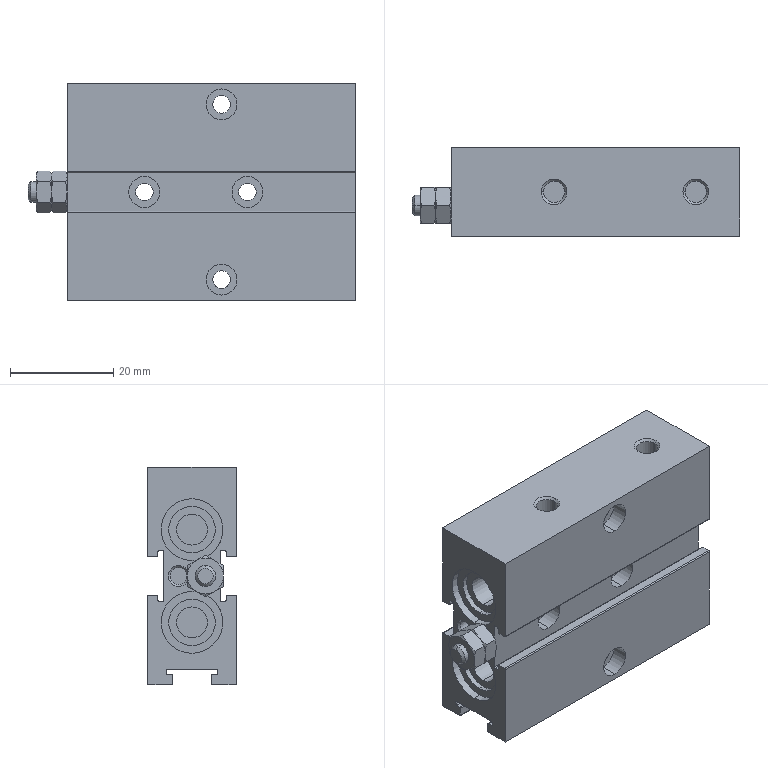Part | SolidWorks | features BaseBody 1 | 1 solid | 190 faces | box 63.5 x 17.2 x 42.3 mm | volume 29328 mm3 | cylinder 82 | plane 72 | cone 36 | commonest cylinder face diameters 0.4 x26 6 x20 3.4 x8 9 x8 12 x8 4.134 x4